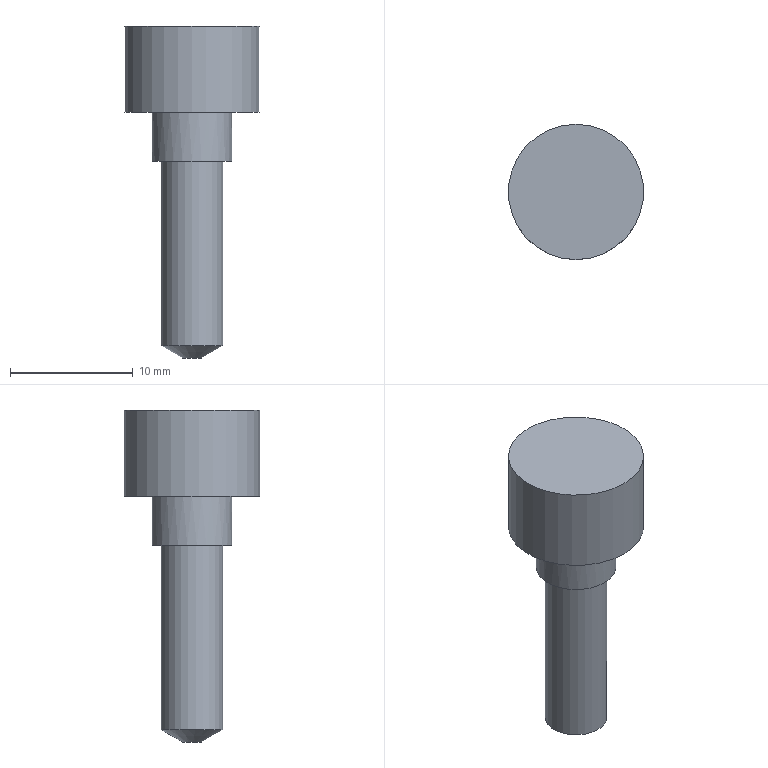Part | STEP file | solid 127 | 1 solid | 8 faces | box 11 x 11 x 27 mm | volume 1102 mm3 | plane 4 | cylinder 3 | cone 1 | commonest cylinder face diameters 5 x1 6.5 x1 11 x1